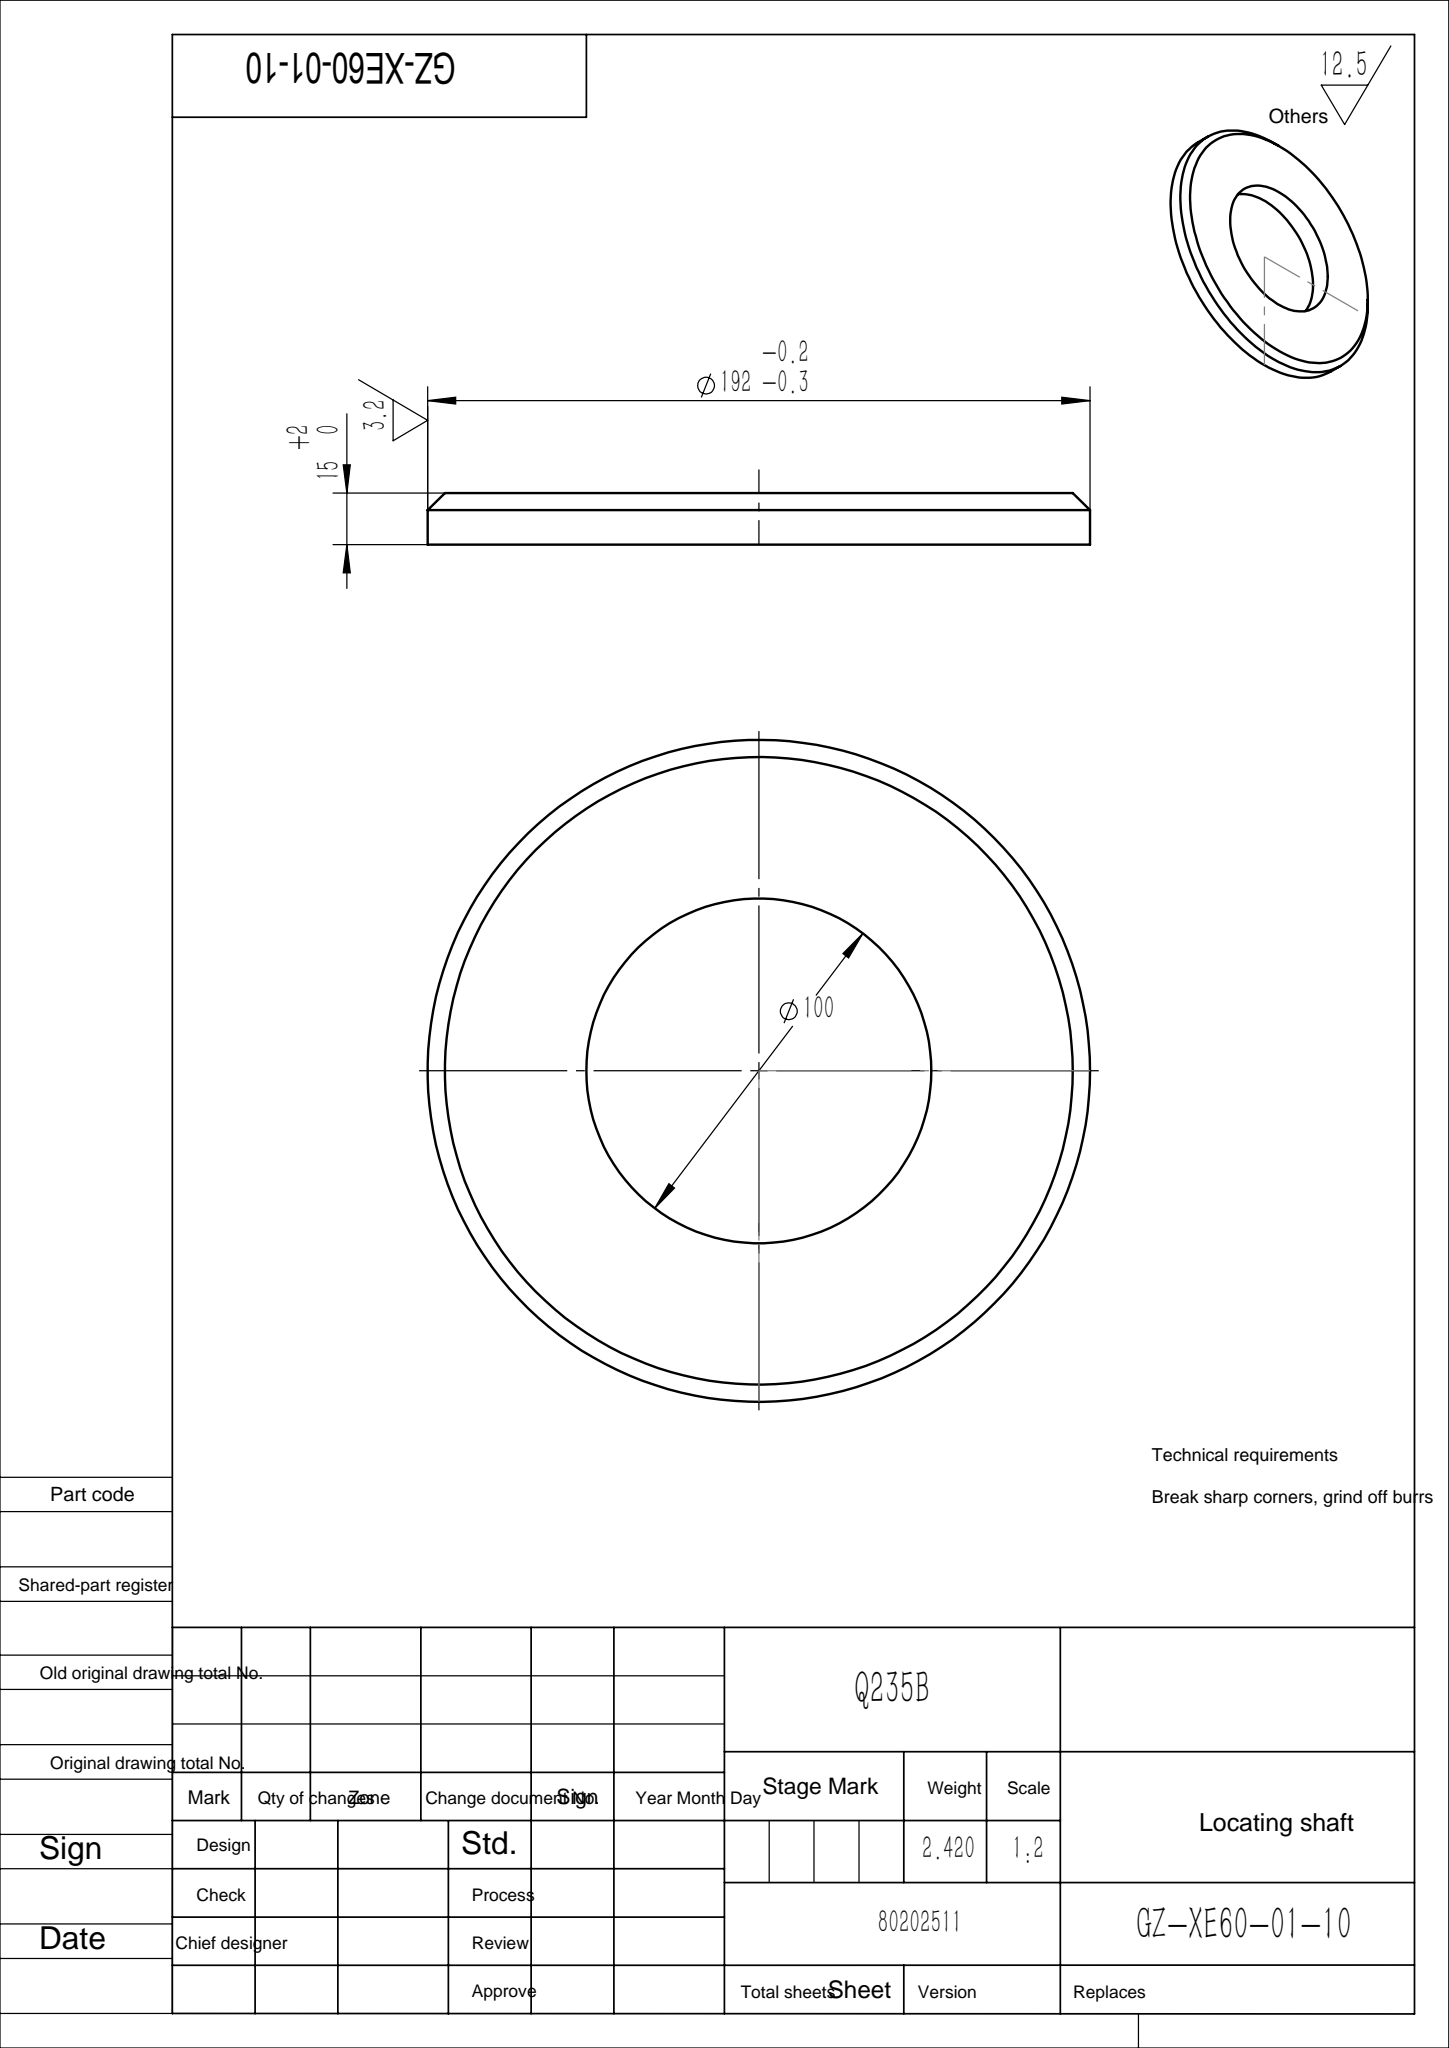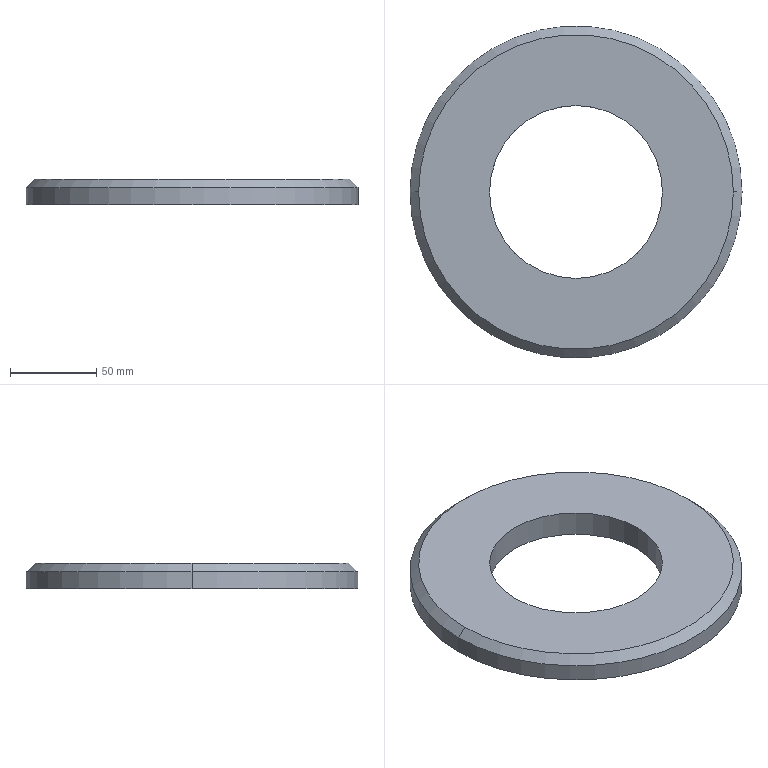Part | SolidWorks | features Chamfer 1, Extrusion 1 | 1 solid | 8 faces | box 192 x 192 x 15 mm | volume 309075 mm3 | cylinder 4 | cone 2 | plane 2 | commonest cylinder face diameters 100 x2 192 x2
STEP:
#1=CARTESIAN_POINT('',(91.,0.,15.));
#2=VERTEX_POINT('',#1);
#3=CARTESIAN_POINT('',(-91.,0.,15.));
#4=VERTEX_POINT('',#3);
#5=CARTESIAN_POINT('',(0.,0.,15.));
#6=DIRECTION('',(0.,0.,1.));
#7=DIRECTION('',(1.,0.,0.));
#8=AXIS2_PLACEMENT_3D('',#5,#6,#7);
#9=CIRCLE('',#8,91.);
#10=EDGE_CURVE('',#2,#4,#9,.T.);
#11=ORIENTED_EDGE('',*,*,#10,.F.);
#12=CARTESIAN_POINT('',(96.,0.,10.));
#13=VERTEX_POINT('',#12);
#14=CARTESIAN_POINT('',(91.,0.,15.));
#15=DIRECTION('',(0.7071,0.,-0.7071));
#16=VECTOR('',#15,1000.);
#17=LINE('',#14,#16);
#18=EDGE_CURVE('',#2,#13,#17,.T.);
#19=ORIENTED_EDGE('',*,*,#18,.T.);
#20=CARTESIAN_POINT('',(-96.,0.,10.));
#21=VERTEX_POINT('',#20);
#22=CARTESIAN_POINT('',(0.,0.,10.));
#23=DIRECTION('',(0.,0.,-1.));
#24=DIRECTION('',(1.,0.,0.));
#25=AXIS2_PLACEMENT_3D('',#22,#23,#24);
#26=CIRCLE('',#25,96.);
#27=EDGE_CURVE('',#21,#13,#26,.T.);
#28=ORIENTED_EDGE('',*,*,#27,.F.);
#29=CARTESIAN_POINT('',(-91.,0.,15.));
#30=DIRECTION('',(-0.7071,0.,-0.7071));
#31=VECTOR('',#30,1000.);
#32=LINE('',#29,#31);
#33=EDGE_CURVE('',#4,#21,#32,.T.);
#34=ORIENTED_EDGE('',*,*,#33,.F.);
#35=EDGE_LOOP('',(#11,#19,#28,#34));
#36=FACE_OUTER_BOUND('',#35,.T.);
#37=CARTESIAN_POINT('',(0.,0.,15.));
#38=DIRECTION('',(0.,0.,-1.));
#39=DIRECTION('',(-1.,0.,0.));
#40=AXIS2_PLACEMENT_3D('',#37,#38,#39);
#41=CONICAL_SURFACE('',#40,91.,0.7854);
#42=ADVANCED_FACE('',(#36),#41,.T.);
#43=CARTESIAN_POINT('',(-50.,0.,15.));
#44=VERTEX_POINT('',#43);
#45=CARTESIAN_POINT('',(50.,0.,15.));
#46=VERTEX_POINT('',#45);
#47=CARTESIAN_POINT('',(0.,0.,15.));
#48=DIRECTION('',(0.,0.,1.));
#49=DIRECTION('',(1.,0.,0.));
#50=AXIS2_PLACEMENT_3D('',#47,#48,#49);
#51=CIRCLE('',#50,50.);
#52=EDGE_CURVE('',#44,#46,#51,.T.);
#53=ORIENTED_EDGE('',*,*,#52,.T.);
#54=CARTESIAN_POINT('',(50.,0.,0.));
#55=VERTEX_POINT('',#54);
#56=CARTESIAN_POINT('',(50.,0.,15.));
#57=DIRECTION('',(0.,0.,-1.));
#58=VECTOR('',#57,1000.);
#59=LINE('',#56,#58);
#60=EDGE_CURVE('',#46,#55,#59,.T.);
#61=ORIENTED_EDGE('',*,*,#60,.T.);
#62=CARTESIAN_POINT('',(-50.,0.,0.));
#63=VERTEX_POINT('',#62);
#64=CARTESIAN_POINT('',(0.,0.,0.));
#65=DIRECTION('',(0.,0.,1.));
#66=DIRECTION('',(1.,0.,0.));
#67=AXIS2_PLACEMENT_3D('',#64,#65,#66);
#68=CIRCLE('',#67,50.);
#69=EDGE_CURVE('',#63,#55,#68,.T.);
#70=ORIENTED_EDGE('',*,*,#69,.F.);
#71=CARTESIAN_POINT('',(-50.,0.,15.));
#72=DIRECTION('',(0.,0.,-1.));
#73=VECTOR('',#72,1000.);
#74=LINE('',#71,#73);
#75=EDGE_CURVE('',#44,#63,#74,.T.);
#76=ORIENTED_EDGE('',*,*,#75,.F.);
#77=EDGE_LOOP('',(#53,#61,#70,#76));
#78=FACE_OUTER_BOUND('',#77,.T.);
#79=CARTESIAN_POINT('',(0.,0.,15.));
#80=DIRECTION('',(0.,0.,-1.));
#81=DIRECTION('',(-1.,0.,0.));
#82=AXIS2_PLACEMENT_3D('',#79,#80,#81);
#83=CYLINDRICAL_SURFACE('',#82,50.);
#84=ADVANCED_FACE('',(#78),#83,.F.);
#85=ORIENTED_EDGE('',*,*,#27,.T.);
#86=CARTESIAN_POINT('',(96.,0.,0.));
#87=VERTEX_POINT('',#86);
#88=CARTESIAN_POINT('',(96.,0.,15.));
#89=DIRECTION('',(0.,0.,-1.));
#90=VECTOR('',#89,1000.);
#91=LINE('',#88,#90);
#92=EDGE_CURVE('',#13,#87,#91,.T.);
#93=ORIENTED_EDGE('',*,*,#92,.T.);
#94=CARTESIAN_POINT('',(-96.,0.,0.));
#95=VERTEX_POINT('',#94);
#96=CARTESIAN_POINT('',(0.,0.,0.));
#97=DIRECTION('',(0.,0.,1.));
#98=DIRECTION('',(1.,0.,0.));
#99=AXIS2_PLACEMENT_3D('',#96,#97,#98);
#100=CIRCLE('',#99,96.);
#101=EDGE_CURVE('',#87,#95,#100,.T.);
#102=ORIENTED_EDGE('',*,*,#101,.T.);
#103=CARTESIAN_POINT('',(-96.,0.,15.));
#104=DIRECTION('',(0.,0.,-1.));
#105=VECTOR('',#104,1000.);
#106=LINE('',#103,#105);
#107=EDGE_CURVE('',#21,#95,#106,.T.);
#108=ORIENTED_EDGE('',*,*,#107,.F.);
#109=EDGE_LOOP('',(#85,#93,#102,#108));
#110=FACE_OUTER_BOUND('',#109,.T.);
#111=CARTESIAN_POINT('',(0.,0.,15.));
#112=DIRECTION('',(0.,0.,-1.));
#113=DIRECTION('',(-1.,0.,0.));
#114=AXIS2_PLACEMENT_3D('',#111,#112,#113);
#115=CYLINDRICAL_SURFACE('',#114,96.);
#116=ADVANCED_FACE('',(#110),#115,.T.);
#117=CARTESIAN_POINT('',(0.,0.,15.));
#118=DIRECTION('',(0.,0.,1.));
#119=DIRECTION('',(1.,0.,0.));
#120=AXIS2_PLACEMENT_3D('',#117,#118,#119);
#121=CIRCLE('',#120,91.);
#122=EDGE_CURVE('',#4,#2,#121,.T.);
#123=ORIENTED_EDGE('',*,*,#122,.T.);
#124=ORIENTED_EDGE('',*,*,#10,.T.);
#125=EDGE_LOOP('',(#123,#124));
#126=FACE_OUTER_BOUND('',#125,.T.);
#127=ORIENTED_EDGE('',*,*,#52,.F.);
#128=CARTESIAN_POINT('',(0.,0.,15.));
#129=DIRECTION('',(0.,0.,1.));
#130=DIRECTION('',(1.,0.,0.));
#131=AXIS2_PLACEMENT_3D('',#128,#129,#130);
#132=CIRCLE('',#131,50.);
#133=EDGE_CURVE('',#46,#44,#132,.T.);
#134=ORIENTED_EDGE('',*,*,#133,.F.);
#135=EDGE_LOOP('',(#127,#134));
#136=FACE_BOUND('',#135,.T.);
#137=CARTESIAN_POINT('',(0.,0.,15.));
#138=DIRECTION('',(0.,0.,1.));
#139=DIRECTION('',(1.,0.,0.));
#140=AXIS2_PLACEMENT_3D('',#137,#138,#139);
#141=PLANE('',#140);
#142=ADVANCED_FACE('',(#126,#136),#141,.T.);
#143=CARTESIAN_POINT('',(0.,0.,0.));
#144=DIRECTION('',(0.,0.,1.));
#145=DIRECTION('',(1.,0.,0.));
#146=AXIS2_PLACEMENT_3D('',#143,#144,#145);
#147=CIRCLE('',#146,96.);
#148=EDGE_CURVE('',#95,#87,#147,.T.);
#149=ORIENTED_EDGE('',*,*,#148,.F.);
#150=ORIENTED_EDGE('',*,*,#101,.F.);
#151=EDGE_LOOP('',(#149,#150));
#152=FACE_OUTER_BOUND('',#151,.T.);
#153=ORIENTED_EDGE('',*,*,#69,.T.);
#154=CARTESIAN_POINT('',(0.,0.,0.));
#155=DIRECTION('',(0.,0.,1.));
#156=DIRECTION('',(1.,0.,0.));
#157=AXIS2_PLACEMENT_3D('',#154,#155,#156);
#158=CIRCLE('',#157,50.);
#159=EDGE_CURVE('',#55,#63,#158,.T.);
#160=ORIENTED_EDGE('',*,*,#159,.T.);
#161=EDGE_LOOP('',(#153,#160));
#162=FACE_BOUND('',#161,.T.);
#163=CARTESIAN_POINT('',(0.,0.,0.));
#164=DIRECTION('',(0.,0.,1.));
#165=DIRECTION('',(1.,0.,0.));
#166=AXIS2_PLACEMENT_3D('',#163,#164,#165);
#167=PLANE('',#166);
#168=ADVANCED_FACE('',(#152,#162),#167,.F.);
#169=ORIENTED_EDGE('',*,*,#92,.F.);
#170=CARTESIAN_POINT('',(0.,0.,10.));
#171=DIRECTION('',(0.,0.,-1.));
#172=DIRECTION('',(1.,0.,0.));
#173=AXIS2_PLACEMENT_3D('',#170,#171,#172);
#174=CIRCLE('',#173,96.);
#175=EDGE_CURVE('',#13,#21,#174,.T.);
#176=ORIENTED_EDGE('',*,*,#175,.T.);
#177=ORIENTED_EDGE('',*,*,#107,.T.);
#178=ORIENTED_EDGE('',*,*,#148,.T.);
#179=EDGE_LOOP('',(#169,#176,#177,#178));
#180=FACE_OUTER_BOUND('',#179,.T.);
#181=CARTESIAN_POINT('',(0.,0.,15.));
#182=DIRECTION('',(0.,0.,-1.));
#183=DIRECTION('',(-1.,0.,0.));
#184=AXIS2_PLACEMENT_3D('',#181,#182,#183);
#185=CYLINDRICAL_SURFACE('',#184,96.);
#186=ADVANCED_FACE('',(#180),#185,.T.);
#187=ORIENTED_EDGE('',*,*,#60,.F.);
#188=ORIENTED_EDGE('',*,*,#133,.T.);
#189=ORIENTED_EDGE('',*,*,#75,.T.);
#190=ORIENTED_EDGE('',*,*,#159,.F.);
#191=EDGE_LOOP('',(#187,#188,#189,#190));
#192=FACE_OUTER_BOUND('',#191,.T.);
#193=CARTESIAN_POINT('',(0.,0.,15.));
#194=DIRECTION('',(0.,0.,-1.));
#195=DIRECTION('',(-1.,0.,0.));
#196=AXIS2_PLACEMENT_3D('',#193,#194,#195);
#197=CYLINDRICAL_SURFACE('',#196,50.);
#198=ADVANCED_FACE('',(#192),#197,.F.);
#199=ORIENTED_EDGE('',*,*,#18,.F.);
#200=ORIENTED_EDGE('',*,*,#122,.F.);
#201=ORIENTED_EDGE('',*,*,#33,.T.);
#202=ORIENTED_EDGE('',*,*,#175,.F.);
#203=EDGE_LOOP('',(#199,#200,#201,#202));
#204=FACE_OUTER_BOUND('',#203,.T.);
#205=CARTESIAN_POINT('',(0.,0.,15.));
#206=DIRECTION('',(0.,0.,-1.));
#207=DIRECTION('',(-1.,0.,0.));
#208=AXIS2_PLACEMENT_3D('',#205,#206,#207);
#209=CONICAL_SURFACE('',#208,91.,0.7854);
#210=ADVANCED_FACE('',(#204),#209,.T.);
#211=CLOSED_SHELL('',(#42,#84,#116,#142,#168,#186,#198,#210));
#212=MANIFOLD_SOLID_BREP('',#211);
#213=CARTESIAN_POINT('',(0.,0.,0.));
#214=DIRECTION('',(0.,0.,1.));
#215=DIRECTION('',(1.,0.,0.));
#216=AXIS2_PLACEMENT_3D('',#213,#214,#215);
#217=(LENGTH_UNIT()NAMED_UNIT(*)SI_UNIT(.MILLI.,.METRE.));
#218=UNCERTAINTY_MEASURE_WITH_UNIT(LENGTH_MEASURE(0.00001),#217,'','');
#219=(NAMED_UNIT(*)PLANE_ANGLE_UNIT()SI_UNIT($,.RADIAN.));
#220=(NAMED_UNIT(*)SI_UNIT($,.STERADIAN.)SOLID_ANGLE_UNIT());
#221=(GEOMETRIC_REPRESENTATION_CONTEXT(3)GLOBAL_UNCERTAINTY_ASSIGNED_CONTEXT((#218))GLOBAL_UNIT_ASSIGNED_CONTEXT((#217,#219,#220))REPRESENTATION_CONTEXT('',''));
#222=ADVANCED_BREP_SHAPE_REPRESENTATION('',(#212,#216),#221);